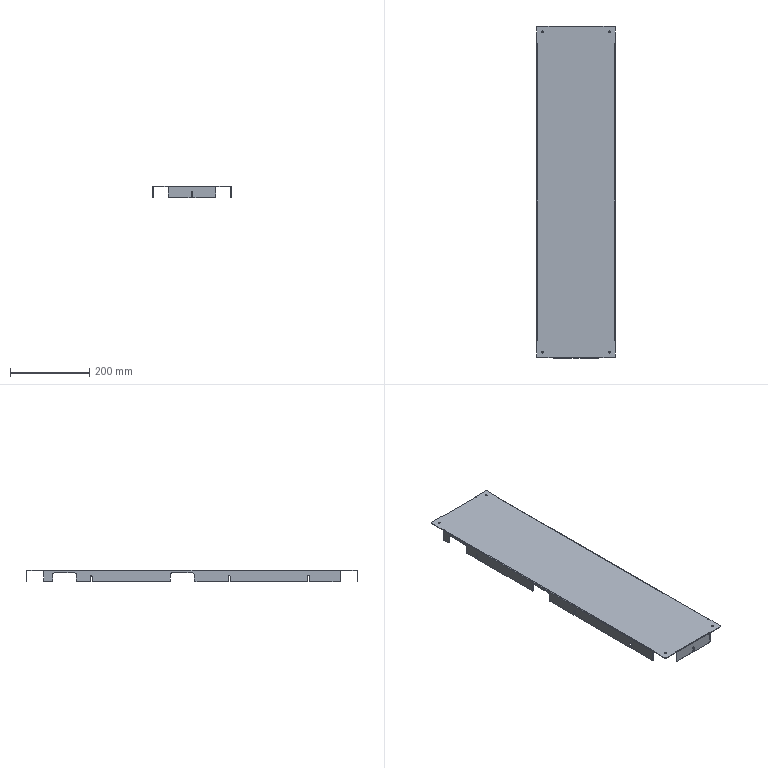Part | STEP file | 1 solid | 158 faces | box 199 x 839 x 30 mm | volume 251918 mm3 | plane 102 | cylinder 56 | commonest cylinder face diameters 4 x18 4.5 x14 5 x8 10 x8 1.2 x4 3.6 x4